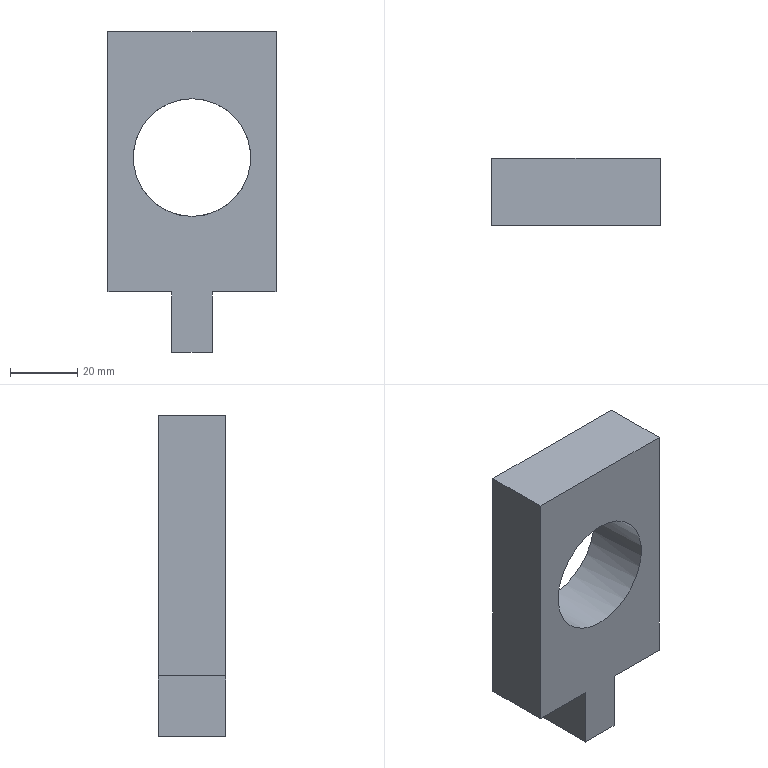Part | STEP file | 冲床-300配套压波_id262_x_t | 1 solid | 11 faces | box 50 x 20 x 95.5 mm | volume 62578 mm3 | plane 10 | cylinder 1 | commonest cylinder face diameters 35 x1
STEP:
#1=CARTESIAN_POINT('',(1124.,-125.,70.));
#2=VERTEX_POINT('',#1);
#3=CARTESIAN_POINT('',(1105.,-125.,70.));
#4=VERTEX_POINT('',#3);
#5=CARTESIAN_POINT('',(1155.,-125.,70.));
#6=DIRECTION('',(-1.,0.,0.));
#7=VECTOR('',#6,1.);
#8=LINE('',#5,#7);
#9=EDGE_CURVE('',#2,#4,#8,.T.);
#10=ORIENTED_EDGE('',*,*,#9,.T.);
#11=CARTESIAN_POINT('',(1105.,-105.,70.));
#12=VERTEX_POINT('',#11);
#13=CARTESIAN_POINT('',(1105.,-105.,70.));
#14=DIRECTION('',(0.,-1.,0.));
#15=VECTOR('',#14,1.);
#16=LINE('',#13,#15);
#17=EDGE_CURVE('',#12,#4,#16,.T.);
#18=ORIENTED_EDGE('',*,*,#17,.F.);
#19=CARTESIAN_POINT('',(1124.,-105.,70.));
#20=VERTEX_POINT('',#19);
#21=CARTESIAN_POINT('',(1105.,-105.,70.));
#22=DIRECTION('',(1.,0.,0.));
#23=VECTOR('',#22,1.);
#24=LINE('',#21,#23);
#25=EDGE_CURVE('',#12,#20,#24,.T.);
#26=ORIENTED_EDGE('',*,*,#25,.T.);
#27=CARTESIAN_POINT('',(1124.,-105.,70.));
#28=DIRECTION('',(0.,-1.,0.));
#29=VECTOR('',#28,1.);
#30=LINE('',#27,#29);
#31=EDGE_CURVE('',#20,#2,#30,.T.);
#32=ORIENTED_EDGE('',*,*,#31,.T.);
#33=EDGE_LOOP('',(#10,#18,#26,#32));
#34=FACE_OUTER_BOUND('',#33,.T.);
#35=CARTESIAN_POINT('',(1105.,-105.,70.));
#36=DIRECTION('',(0.,0.,1.));
#37=DIRECTION('',(1.,0.,0.));
#38=AXIS2_PLACEMENT_3D('',#35,#36,#37);
#39=PLANE('',#38);
#40=ADVANCED_FACE('',(#34),#39,.F.);
#41=CARTESIAN_POINT('',(1105.,-105.,147.5));
#42=VERTEX_POINT('',#41);
#43=CARTESIAN_POINT('',(1105.,-125.,147.5));
#44=VERTEX_POINT('',#43);
#45=CARTESIAN_POINT('',(1105.,-125.,147.5));
#46=DIRECTION('',(0.,-1.,0.));
#47=VECTOR('',#46,1.);
#48=LINE('',#45,#47);
#49=EDGE_CURVE('',#42,#44,#48,.T.);
#50=ORIENTED_EDGE('',*,*,#49,.F.);
#51=CARTESIAN_POINT('',(1105.,-105.,150.));
#52=DIRECTION('',(0.,0.,-1.));
#53=VECTOR('',#52,1.);
#54=LINE('',#51,#53);
#55=EDGE_CURVE('',#42,#12,#54,.T.);
#56=ORIENTED_EDGE('',*,*,#55,.T.);
#57=ORIENTED_EDGE('',*,*,#17,.T.);
#58=CARTESIAN_POINT('',(1105.,-125.,150.));
#59=DIRECTION('',(0.,0.,-1.));
#60=VECTOR('',#59,1.);
#61=LINE('',#58,#60);
#62=EDGE_CURVE('',#44,#4,#61,.T.);
#63=ORIENTED_EDGE('',*,*,#62,.F.);
#64=EDGE_LOOP('',(#50,#56,#57,#63));
#65=FACE_OUTER_BOUND('',#64,.T.);
#66=CARTESIAN_POINT('',(1105.,-125.,150.));
#67=DIRECTION('',(1.,0.,0.));
#68=DIRECTION('',(0.,0.,-1.));
#69=AXIS2_PLACEMENT_3D('',#66,#67,#68);
#70=PLANE('',#69);
#71=ADVANCED_FACE('',(#65),#70,.F.);
#72=CARTESIAN_POINT('',(1155.,-125.,147.5));
#73=VERTEX_POINT('',#72);
#74=CARTESIAN_POINT('',(1155.,-125.,147.5));
#75=DIRECTION('',(1.,0.,0.));
#76=VECTOR('',#75,1.);
#77=LINE('',#74,#76);
#78=EDGE_CURVE('',#44,#73,#77,.T.);
#79=ORIENTED_EDGE('',*,*,#78,.F.);
#80=ORIENTED_EDGE('',*,*,#62,.T.);
#81=ORIENTED_EDGE('',*,*,#9,.F.);
#82=CARTESIAN_POINT('',(1124.,-125.,52.));
#83=VERTEX_POINT('',#82);
#84=CARTESIAN_POINT('',(1124.,-125.,78.));
#85=DIRECTION('',(0.,0.,1.));
#86=VECTOR('',#85,1.);
#87=LINE('',#84,#86);
#88=EDGE_CURVE('',#83,#2,#87,.T.);
#89=ORIENTED_EDGE('',*,*,#88,.F.);
#90=CARTESIAN_POINT('',(1136.,-125.,52.));
#91=VERTEX_POINT('',#90);
#92=CARTESIAN_POINT('',(1155.,-125.,52.));
#93=DIRECTION('',(1.,0.,0.));
#94=VECTOR('',#93,1.);
#95=LINE('',#92,#94);
#96=EDGE_CURVE('',#83,#91,#95,.T.);
#97=ORIENTED_EDGE('',*,*,#96,.T.);
#98=CARTESIAN_POINT('',(1136.,-125.,70.));
#99=VERTEX_POINT('',#98);
#100=CARTESIAN_POINT('',(1136.,-125.,46.));
#101=DIRECTION('',(0.,0.,-1.));
#102=VECTOR('',#101,1.);
#103=LINE('',#100,#102);
#104=EDGE_CURVE('',#99,#91,#103,.T.);
#105=ORIENTED_EDGE('',*,*,#104,.F.);
#106=CARTESIAN_POINT('',(1155.,-125.,70.));
#107=VERTEX_POINT('',#106);
#108=CARTESIAN_POINT('',(1155.,-125.,70.));
#109=DIRECTION('',(-1.,0.,0.));
#110=VECTOR('',#109,1.);
#111=LINE('',#108,#110);
#112=EDGE_CURVE('',#107,#99,#111,.T.);
#113=ORIENTED_EDGE('',*,*,#112,.F.);
#114=CARTESIAN_POINT('',(1155.,-125.,150.));
#115=DIRECTION('',(0.,0.,-1.));
#116=VECTOR('',#115,1.);
#117=LINE('',#114,#116);
#118=EDGE_CURVE('',#73,#107,#117,.T.);
#119=ORIENTED_EDGE('',*,*,#118,.F.);
#120=EDGE_LOOP('',(#79,#80,#81,#89,#97,#105,#113,#119));
#121=FACE_BOUND('',#120,.T.);
#122=CARTESIAN_POINT('',(1130.,-125.,92.5));
#123=VERTEX_POINT('',#122);
#124=CARTESIAN_POINT('',(1130.,-125.,110.));
#125=DIRECTION('',(0.,-1.,0.));
#126=DIRECTION('',(0.,0.,-1.));
#127=AXIS2_PLACEMENT_3D('',#124,#125,#126);
#128=CIRCLE('',#127,17.5);
#129=EDGE_CURVE('',#123,#123,#128,.T.);
#130=ORIENTED_EDGE('',*,*,#129,.F.);
#131=EDGE_LOOP('',(#130));
#132=FACE_BOUND('',#131,.T.);
#133=CARTESIAN_POINT('',(1155.,-125.,150.));
#134=DIRECTION('',(0.,1.,0.));
#135=DIRECTION('',(0.,0.,-1.));
#136=AXIS2_PLACEMENT_3D('',#133,#134,#135);
#137=PLANE('',#136);
#138=ADVANCED_FACE('',(#121,#132),#137,.F.);
#139=CARTESIAN_POINT('',(1155.,-105.,147.5));
#140=VERTEX_POINT('',#139);
#141=CARTESIAN_POINT('',(1105.,-105.,147.5));
#142=DIRECTION('',(-1.,0.,0.));
#143=VECTOR('',#142,1.);
#144=LINE('',#141,#143);
#145=EDGE_CURVE('',#140,#42,#144,.T.);
#146=ORIENTED_EDGE('',*,*,#145,.F.);
#147=CARTESIAN_POINT('',(1155.,-105.,70.));
#148=VERTEX_POINT('',#147);
#149=CARTESIAN_POINT('',(1155.,-105.,150.));
#150=DIRECTION('',(0.,0.,-1.));
#151=VECTOR('',#150,1.);
#152=LINE('',#149,#151);
#153=EDGE_CURVE('',#140,#148,#152,.T.);
#154=ORIENTED_EDGE('',*,*,#153,.T.);
#155=CARTESIAN_POINT('',(1136.,-105.,70.));
#156=VERTEX_POINT('',#155);
#157=CARTESIAN_POINT('',(1105.,-105.,70.));
#158=DIRECTION('',(1.,0.,0.));
#159=VECTOR('',#158,1.);
#160=LINE('',#157,#159);
#161=EDGE_CURVE('',#156,#148,#160,.T.);
#162=ORIENTED_EDGE('',*,*,#161,.F.);
#163=CARTESIAN_POINT('',(1136.,-105.,52.));
#164=VERTEX_POINT('',#163);
#165=CARTESIAN_POINT('',(1136.,-105.,150.));
#166=DIRECTION('',(0.,0.,1.));
#167=VECTOR('',#166,1.);
#168=LINE('',#165,#167);
#169=EDGE_CURVE('',#164,#156,#168,.T.);
#170=ORIENTED_EDGE('',*,*,#169,.F.);
#171=CARTESIAN_POINT('',(1124.,-105.,52.));
#172=VERTEX_POINT('',#171);
#173=CARTESIAN_POINT('',(1155.,-105.,52.));
#174=DIRECTION('',(1.,0.,0.));
#175=VECTOR('',#174,1.);
#176=LINE('',#173,#175);
#177=EDGE_CURVE('',#172,#164,#176,.T.);
#178=ORIENTED_EDGE('',*,*,#177,.F.);
#179=CARTESIAN_POINT('',(1124.,-105.,150.));
#180=DIRECTION('',(0.,0.,-1.));
#181=VECTOR('',#180,1.);
#182=LINE('',#179,#181);
#183=EDGE_CURVE('',#20,#172,#182,.T.);
#184=ORIENTED_EDGE('',*,*,#183,.F.);
#185=ORIENTED_EDGE('',*,*,#25,.F.);
#186=ORIENTED_EDGE('',*,*,#55,.F.);
#187=EDGE_LOOP('',(#146,#154,#162,#170,#178,#184,#185,#186));
#188=FACE_BOUND('',#187,.T.);
#189=CARTESIAN_POINT('',(1130.,-105.,127.5));
#190=VERTEX_POINT('',#189);
#191=CARTESIAN_POINT('',(1130.,-105.,110.));
#192=DIRECTION('',(0.,1.,0.));
#193=DIRECTION('',(0.,0.,1.));
#194=AXIS2_PLACEMENT_3D('',#191,#192,#193);
#195=CIRCLE('',#194,17.5);
#196=EDGE_CURVE('',#190,#190,#195,.T.);
#197=ORIENTED_EDGE('',*,*,#196,.F.);
#198=EDGE_LOOP('',(#197));
#199=FACE_BOUND('',#198,.T.);
#200=CARTESIAN_POINT('',(1105.,-105.,150.));
#201=DIRECTION('',(0.,-1.,0.));
#202=DIRECTION('',(0.,0.,1.));
#203=AXIS2_PLACEMENT_3D('',#200,#201,#202);
#204=PLANE('',#203);
#205=ADVANCED_FACE('',(#188,#199),#204,.F.);
#206=CARTESIAN_POINT('',(1155.,-105.,147.5));
#207=DIRECTION('',(0.,1.,0.));
#208=VECTOR('',#207,1.);
#209=LINE('',#206,#208);
#210=EDGE_CURVE('',#73,#140,#209,.T.);
#211=ORIENTED_EDGE('',*,*,#210,.F.);
#212=ORIENTED_EDGE('',*,*,#118,.T.);
#213=CARTESIAN_POINT('',(1155.,-105.,70.));
#214=DIRECTION('',(0.,-1.,0.));
#215=VECTOR('',#214,1.);
#216=LINE('',#213,#215);
#217=EDGE_CURVE('',#148,#107,#216,.T.);
#218=ORIENTED_EDGE('',*,*,#217,.F.);
#219=ORIENTED_EDGE('',*,*,#153,.F.);
#220=EDGE_LOOP('',(#211,#212,#218,#219));
#221=FACE_OUTER_BOUND('',#220,.T.);
#222=CARTESIAN_POINT('',(1155.,-105.,150.));
#223=DIRECTION('',(-1.,0.,0.));
#224=DIRECTION('',(0.,0.,1.));
#225=AXIS2_PLACEMENT_3D('',#222,#223,#224);
#226=PLANE('',#225);
#227=ADVANCED_FACE('',(#221),#226,.F.);
#228=ORIENTED_EDGE('',*,*,#129,.T.);
#229=EDGE_LOOP('',(#228));
#230=FACE_BOUND('',#229,.T.);
#231=ORIENTED_EDGE('',*,*,#196,.T.);
#232=EDGE_LOOP('',(#231));
#233=FACE_BOUND('',#232,.T.);
#234=CARTESIAN_POINT('',(1130.,25.15,110.));
#235=DIRECTION('',(0.,-1.,0.));
#236=DIRECTION('',(0.,0.,1.));
#237=AXIS2_PLACEMENT_3D('',#234,#235,#236);
#238=CYLINDRICAL_SURFACE('',#237,17.5);
#239=ADVANCED_FACE('',(#230,#233),#238,.F.);
#240=ORIENTED_EDGE('',*,*,#161,.T.);
#241=ORIENTED_EDGE('',*,*,#217,.T.);
#242=ORIENTED_EDGE('',*,*,#112,.T.);
#243=CARTESIAN_POINT('',(1136.,-105.,70.));
#244=DIRECTION('',(0.,1.,0.));
#245=VECTOR('',#244,1.);
#246=LINE('',#243,#245);
#247=EDGE_CURVE('',#99,#156,#246,.T.);
#248=ORIENTED_EDGE('',*,*,#247,.T.);
#249=EDGE_LOOP('',(#240,#241,#242,#248));
#250=FACE_OUTER_BOUND('',#249,.T.);
#251=CARTESIAN_POINT('',(1105.,-105.,70.));
#252=DIRECTION('',(0.,0.,1.));
#253=DIRECTION('',(1.,0.,0.));
#254=AXIS2_PLACEMENT_3D('',#251,#252,#253);
#255=PLANE('',#254);
#256=ADVANCED_FACE('',(#250),#255,.F.);
#257=ORIENTED_EDGE('',*,*,#183,.T.);
#258=CARTESIAN_POINT('',(1124.,-125.,52.));
#259=DIRECTION('',(0.,-1.,0.));
#260=VECTOR('',#259,1.);
#261=LINE('',#258,#260);
#262=EDGE_CURVE('',#172,#83,#261,.T.);
#263=ORIENTED_EDGE('',*,*,#262,.T.);
#264=ORIENTED_EDGE('',*,*,#88,.T.);
#265=ORIENTED_EDGE('',*,*,#31,.F.);
#266=EDGE_LOOP('',(#257,#263,#264,#265));
#267=FACE_OUTER_BOUND('',#266,.T.);
#268=CARTESIAN_POINT('',(1124.,-125.,78.));
#269=DIRECTION('',(-1.,0.,0.));
#270=DIRECTION('',(0.,0.,1.));
#271=AXIS2_PLACEMENT_3D('',#268,#269,#270);
#272=PLANE('',#271);
#273=ADVANCED_FACE('',(#267),#272,.T.);
#274=ORIENTED_EDGE('',*,*,#247,.F.);
#275=ORIENTED_EDGE('',*,*,#104,.T.);
#276=CARTESIAN_POINT('',(1136.,-105.,52.));
#277=DIRECTION('',(0.,-1.,0.));
#278=VECTOR('',#277,1.);
#279=LINE('',#276,#278);
#280=EDGE_CURVE('',#164,#91,#279,.T.);
#281=ORIENTED_EDGE('',*,*,#280,.F.);
#282=ORIENTED_EDGE('',*,*,#169,.T.);
#283=EDGE_LOOP('',(#274,#275,#281,#282));
#284=FACE_OUTER_BOUND('',#283,.T.);
#285=CARTESIAN_POINT('',(1136.,-125.,46.));
#286=DIRECTION('',(1.,0.,0.));
#287=DIRECTION('',(0.,0.,-1.));
#288=AXIS2_PLACEMENT_3D('',#285,#286,#287);
#289=PLANE('',#288);
#290=ADVANCED_FACE('',(#284),#289,.T.);
#291=ORIENTED_EDGE('',*,*,#177,.T.);
#292=ORIENTED_EDGE('',*,*,#280,.T.);
#293=ORIENTED_EDGE('',*,*,#96,.F.);
#294=ORIENTED_EDGE('',*,*,#262,.F.);
#295=EDGE_LOOP('',(#291,#292,#293,#294));
#296=FACE_OUTER_BOUND('',#295,.T.);
#297=CARTESIAN_POINT('',(1155.,-105.,52.));
#298=DIRECTION('',(0.,0.,-1.));
#299=DIRECTION('',(-1.,0.,0.));
#300=AXIS2_PLACEMENT_3D('',#297,#298,#299);
#301=PLANE('',#300);
#302=ADVANCED_FACE('',(#296),#301,.T.);
#303=ORIENTED_EDGE('',*,*,#49,.T.);
#304=ORIENTED_EDGE('',*,*,#78,.T.);
#305=ORIENTED_EDGE('',*,*,#210,.T.);
#306=ORIENTED_EDGE('',*,*,#145,.T.);
#307=EDGE_LOOP('',(#303,#304,#305,#306));
#308=FACE_OUTER_BOUND('',#307,.T.);
#309=CARTESIAN_POINT('',(1130.,-110.075,147.5));
#310=DIRECTION('',(0.,0.,-1.));
#311=DIRECTION('',(-1.,0.,0.));
#312=AXIS2_PLACEMENT_3D('',#309,#310,#311);
#313=PLANE('',#312);
#314=ADVANCED_FACE('',(#308),#313,.F.);
#315=CLOSED_SHELL('',(#40,#71,#138,#205,#227,#239,#256,#273,#290,#302,#314));
#316=MANIFOLD_SOLID_BREP('',#315);
#317=(LENGTH_UNIT()NAMED_UNIT(*)SI_UNIT(.MILLI.,.METRE.));
#318=UNCERTAINTY_MEASURE_WITH_UNIT(LENGTH_MEASURE(0.00002),#317,'','');
#319=(NAMED_UNIT(*)PLANE_ANGLE_UNIT()SI_UNIT($,.RADIAN.));
#320=PLANE_ANGLE_MEASURE_WITH_UNIT(PLANE_ANGLE_MEASURE(0.01745),#319);
#321=DIMENSIONAL_EXPONENTS(0.,0.,0.,0.,0.,0.,0.);
#322=(CONVERSION_BASED_UNIT('DEGREE',#320)NAMED_UNIT(#321)PLANE_ANGLE_UNIT());
#323=(NAMED_UNIT(*)SI_UNIT($,.STERADIAN.)SOLID_ANGLE_UNIT());
#324=(GEOMETRIC_REPRESENTATION_CONTEXT(3)GLOBAL_UNCERTAINTY_ASSIGNED_CONTEXT((#318))GLOBAL_UNIT_ASSIGNED_CONTEXT((#317,#322,#323))REPRESENTATION_CONTEXT('',''));
#325=ADVANCED_BREP_SHAPE_REPRESENTATION('',(#316),#324);